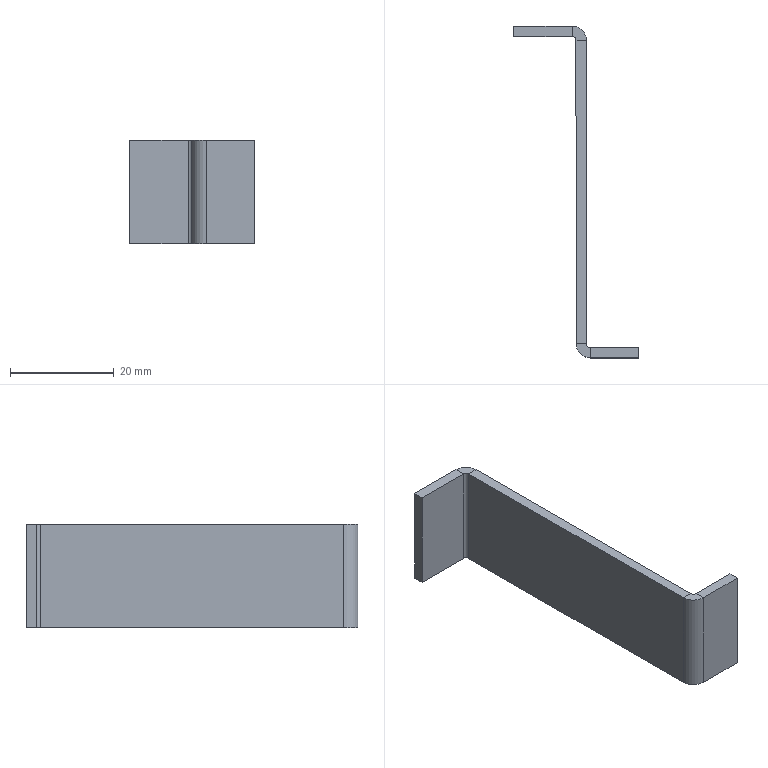Part | SolidWorks | features FlatPattern 1, SMBaseFlange 1, SheetMetal 1 | 1 solid | 22 faces | box 24 x 64 x 20 mm | volume 3380 mm3 | plane 18 | cylinder 4 | commonest cylinder face diameters 1.473 x2 5.473 x2
STEP:
#1=CARTESIAN_POINT('',(14.,-2.737,10.));
#2=VERTEX_POINT('',#1);
#3=CARTESIAN_POINT('',(12.,-2.737,10.));
#4=VERTEX_POINT('',#3);
#5=CARTESIAN_POINT('',(14.,-2.737,10.));
#6=DIRECTION('',(-1.,0.,0.));
#7=VECTOR('',#6,1000.);
#8=LINE('',#5,#7);
#9=EDGE_CURVE('',#2,#4,#8,.T.);
#10=ORIENTED_EDGE('',*,*,#9,.F.);
#11=CARTESIAN_POINT('',(11.263,0.,10.));
#12=VERTEX_POINT('',#11);
#13=CARTESIAN_POINT('',(11.263,-2.737,10.));
#14=DIRECTION('',(0.,0.,-1.));
#15=DIRECTION('',(1.,0.,0.));
#16=AXIS2_PLACEMENT_3D('',#13,#14,#15);
#17=CIRCLE('',#16,2.737);
#18=EDGE_CURVE('',#12,#2,#17,.T.);
#19=ORIENTED_EDGE('',*,*,#18,.F.);
#20=CARTESIAN_POINT('',(11.263,-2.,10.));
#21=VERTEX_POINT('',#20);
#22=CARTESIAN_POINT('',(11.263,-2.,10.));
#23=DIRECTION('',(0.,1.,0.));
#24=VECTOR('',#23,1000.);
#25=LINE('',#22,#24);
#26=EDGE_CURVE('',#21,#12,#25,.T.);
#27=ORIENTED_EDGE('',*,*,#26,.F.);
#28=CARTESIAN_POINT('',(11.263,-2.737,10.));
#29=DIRECTION('',(0.,0.,-1.));
#30=DIRECTION('',(1.,0.,0.));
#31=AXIS2_PLACEMENT_3D('',#28,#29,#30);
#32=CIRCLE('',#31,0.7366);
#33=EDGE_CURVE('',#21,#4,#32,.T.);
#34=ORIENTED_EDGE('',*,*,#33,.T.);
#35=EDGE_LOOP('',(#10,#19,#27,#34));
#36=FACE_OUTER_BOUND('',#35,.T.);
#37=CARTESIAN_POINT('',(14.,-2.737,10.));
#38=DIRECTION('',(0.,0.,1.));
#39=DIRECTION('',(1.,0.,0.));
#40=AXIS2_PLACEMENT_3D('',#37,#38,#39);
#41=PLANE('',#40);
#42=ADVANCED_FACE('',(#36),#41,.T.);
#43=CARTESIAN_POINT('',(14.,-61.263,10.));
#44=VERTEX_POINT('',#43);
#45=CARTESIAN_POINT('',(14.,0.,10.));
#46=DIRECTION('',(0.,-1.,0.));
#47=VECTOR('',#46,1000.);
#48=LINE('',#45,#47);
#49=EDGE_CURVE('',#2,#44,#48,.T.);
#50=ORIENTED_EDGE('',*,*,#49,.F.);
#51=ORIENTED_EDGE('',*,*,#9,.T.);
#52=CARTESIAN_POINT('',(12.,-61.263,10.));
#53=VERTEX_POINT('',#52);
#54=CARTESIAN_POINT('',(12.,0.,10.));
#55=DIRECTION('',(0.,-1.,0.));
#56=VECTOR('',#55,1000.);
#57=LINE('',#54,#56);
#58=EDGE_CURVE('',#4,#53,#57,.T.);
#59=ORIENTED_EDGE('',*,*,#58,.T.);
#60=CARTESIAN_POINT('',(12.,-61.263,10.));
#61=DIRECTION('',(1.,0.,0.));
#62=VECTOR('',#61,1000.);
#63=LINE('',#60,#62);
#64=EDGE_CURVE('',#53,#44,#63,.T.);
#65=ORIENTED_EDGE('',*,*,#64,.T.);
#66=EDGE_LOOP('',(#50,#51,#59,#65));
#67=FACE_OUTER_BOUND('',#66,.T.);
#68=CARTESIAN_POINT('',(11.263,-2.,10.));
#69=DIRECTION('',(0.,0.,1.));
#70=DIRECTION('',(1.,0.,0.));
#71=AXIS2_PLACEMENT_3D('',#68,#69,#70);
#72=PLANE('',#71);
#73=ADVANCED_FACE('',(#67),#72,.T.);
#74=CARTESIAN_POINT('',(11.263,0.,-10.));
#75=VERTEX_POINT('',#74);
#76=CARTESIAN_POINT('',(11.263,-2.,-10.));
#77=VERTEX_POINT('',#76);
#78=CARTESIAN_POINT('',(11.263,0.,-10.));
#79=DIRECTION('',(0.,-1.,0.));
#80=VECTOR('',#79,1000.);
#81=LINE('',#78,#80);
#82=EDGE_CURVE('',#75,#77,#81,.T.);
#83=ORIENTED_EDGE('',*,*,#82,.F.);
#84=CARTESIAN_POINT('',(14.,-2.737,-10.));
#85=VERTEX_POINT('',#84);
#86=CARTESIAN_POINT('',(11.263,-2.737,-10.));
#87=DIRECTION('',(0.,0.,-1.));
#88=DIRECTION('',(1.,0.,0.));
#89=AXIS2_PLACEMENT_3D('',#86,#87,#88);
#90=CIRCLE('',#89,2.737);
#91=EDGE_CURVE('',#75,#85,#90,.T.);
#92=ORIENTED_EDGE('',*,*,#91,.T.);
#93=CARTESIAN_POINT('',(12.,-2.737,-10.));
#94=VERTEX_POINT('',#93);
#95=CARTESIAN_POINT('',(12.,-2.737,-10.));
#96=DIRECTION('',(1.,0.,0.));
#97=VECTOR('',#96,1000.);
#98=LINE('',#95,#97);
#99=EDGE_CURVE('',#94,#85,#98,.T.);
#100=ORIENTED_EDGE('',*,*,#99,.F.);
#101=CARTESIAN_POINT('',(11.263,-2.737,-10.));
#102=DIRECTION('',(0.,0.,-1.));
#103=DIRECTION('',(1.,0.,0.));
#104=AXIS2_PLACEMENT_3D('',#101,#102,#103);
#105=CIRCLE('',#104,0.7366);
#106=EDGE_CURVE('',#77,#94,#105,.T.);
#107=ORIENTED_EDGE('',*,*,#106,.F.);
#108=EDGE_LOOP('',(#83,#92,#100,#107));
#109=FACE_OUTER_BOUND('',#108,.T.);
#110=CARTESIAN_POINT('',(11.263,0.,-10.));
#111=DIRECTION('',(0.,0.,-1.));
#112=DIRECTION('',(-1.,0.,0.));
#113=AXIS2_PLACEMENT_3D('',#110,#111,#112);
#114=PLANE('',#113);
#115=ADVANCED_FACE('',(#109),#114,.T.);
#116=CARTESIAN_POINT('',(0.,0.,-10.));
#117=VERTEX_POINT('',#116);
#118=CARTESIAN_POINT('',(0.,0.,-10.));
#119=DIRECTION('',(1.,0.,0.));
#120=VECTOR('',#119,1000.);
#121=LINE('',#118,#120);
#122=EDGE_CURVE('',#117,#75,#121,.T.);
#123=ORIENTED_EDGE('',*,*,#122,.T.);
#124=ORIENTED_EDGE('',*,*,#82,.T.);
#125=CARTESIAN_POINT('',(0.,-2.,-10.));
#126=VERTEX_POINT('',#125);
#127=CARTESIAN_POINT('',(0.,-2.,-10.));
#128=DIRECTION('',(1.,0.,0.));
#129=VECTOR('',#128,1000.);
#130=LINE('',#127,#129);
#131=EDGE_CURVE('',#126,#77,#130,.T.);
#132=ORIENTED_EDGE('',*,*,#131,.F.);
#133=CARTESIAN_POINT('',(0.,-2.,-10.));
#134=DIRECTION('',(0.,1.,0.));
#135=VECTOR('',#134,1000.);
#136=LINE('',#133,#135);
#137=EDGE_CURVE('',#126,#117,#136,.T.);
#138=ORIENTED_EDGE('',*,*,#137,.T.);
#139=EDGE_LOOP('',(#123,#124,#132,#138));
#140=FACE_OUTER_BOUND('',#139,.T.);
#141=CARTESIAN_POINT('',(12.,-2.737,-10.));
#142=DIRECTION('',(0.,0.,-1.));
#143=DIRECTION('',(-1.,0.,0.));
#144=AXIS2_PLACEMENT_3D('',#141,#142,#143);
#145=PLANE('',#144);
#146=ADVANCED_FACE('',(#140),#145,.T.);
#147=CARTESIAN_POINT('',(14.737,-62.,10.));
#148=VERTEX_POINT('',#147);
#149=CARTESIAN_POINT('',(14.737,-64.,10.));
#150=VERTEX_POINT('',#149);
#151=CARTESIAN_POINT('',(14.737,-62.,10.));
#152=DIRECTION('',(0.,-1.,0.));
#153=VECTOR('',#152,1000.);
#154=LINE('',#151,#153);
#155=EDGE_CURVE('',#148,#150,#154,.T.);
#156=ORIENTED_EDGE('',*,*,#155,.F.);
#157=CARTESIAN_POINT('',(14.737,-61.263,10.));
#158=DIRECTION('',(0.,0.,1.));
#159=DIRECTION('',(-1.,0.,0.));
#160=AXIS2_PLACEMENT_3D('',#157,#158,#159);
#161=CIRCLE('',#160,0.7366);
#162=EDGE_CURVE('',#44,#148,#161,.T.);
#163=ORIENTED_EDGE('',*,*,#162,.F.);
#164=ORIENTED_EDGE('',*,*,#64,.F.);
#165=CARTESIAN_POINT('',(14.737,-61.263,10.));
#166=DIRECTION('',(0.,0.,1.));
#167=DIRECTION('',(1.,0.,0.));
#168=AXIS2_PLACEMENT_3D('',#165,#166,#167);
#169=CIRCLE('',#168,2.737);
#170=EDGE_CURVE('',#53,#150,#169,.T.);
#171=ORIENTED_EDGE('',*,*,#170,.T.);
#172=EDGE_LOOP('',(#156,#163,#164,#171));
#173=FACE_OUTER_BOUND('',#172,.T.);
#174=CARTESIAN_POINT('',(14.737,-62.,10.));
#175=DIRECTION('',(0.,0.,1.));
#176=DIRECTION('',(1.,0.,0.));
#177=AXIS2_PLACEMENT_3D('',#174,#175,#176);
#178=PLANE('',#177);
#179=ADVANCED_FACE('',(#173),#178,.T.);
#180=CARTESIAN_POINT('',(24.,-62.,10.));
#181=VERTEX_POINT('',#180);
#182=CARTESIAN_POINT('',(14.,-62.,10.));
#183=DIRECTION('',(1.,0.,0.));
#184=VECTOR('',#183,1000.);
#185=LINE('',#182,#184);
#186=EDGE_CURVE('',#148,#181,#185,.T.);
#187=ORIENTED_EDGE('',*,*,#186,.F.);
#188=ORIENTED_EDGE('',*,*,#155,.T.);
#189=CARTESIAN_POINT('',(24.,-64.,10.));
#190=VERTEX_POINT('',#189);
#191=CARTESIAN_POINT('',(14.,-64.,10.));
#192=DIRECTION('',(1.,0.,0.));
#193=VECTOR('',#192,1000.);
#194=LINE('',#191,#193);
#195=EDGE_CURVE('',#150,#190,#194,.T.);
#196=ORIENTED_EDGE('',*,*,#195,.T.);
#197=CARTESIAN_POINT('',(24.,-62.,10.));
#198=DIRECTION('',(0.,-1.,0.));
#199=VECTOR('',#198,1000.);
#200=LINE('',#197,#199);
#201=EDGE_CURVE('',#181,#190,#200,.T.);
#202=ORIENTED_EDGE('',*,*,#201,.F.);
#203=EDGE_LOOP('',(#187,#188,#196,#202));
#204=FACE_OUTER_BOUND('',#203,.T.);
#205=CARTESIAN_POINT('',(12.,-61.263,10.));
#206=DIRECTION('',(0.,0.,1.));
#207=DIRECTION('',(1.,0.,0.));
#208=AXIS2_PLACEMENT_3D('',#205,#206,#207);
#209=PLANE('',#208);
#210=ADVANCED_FACE('',(#204),#209,.T.);
#211=CARTESIAN_POINT('',(14.,-61.263,-10.));
#212=VERTEX_POINT('',#211);
#213=CARTESIAN_POINT('',(12.,-61.263,-10.));
#214=VERTEX_POINT('',#213);
#215=CARTESIAN_POINT('',(14.,-61.263,-10.));
#216=DIRECTION('',(-1.,0.,0.));
#217=VECTOR('',#216,1000.);
#218=LINE('',#215,#217);
#219=EDGE_CURVE('',#212,#214,#218,.T.);
#220=ORIENTED_EDGE('',*,*,#219,.F.);
#221=CARTESIAN_POINT('',(14.737,-62.,-10.));
#222=VERTEX_POINT('',#221);
#223=CARTESIAN_POINT('',(14.737,-61.263,-10.));
#224=DIRECTION('',(0.,0.,1.));
#225=DIRECTION('',(-1.,0.,0.));
#226=AXIS2_PLACEMENT_3D('',#223,#224,#225);
#227=CIRCLE('',#226,0.7366);
#228=EDGE_CURVE('',#212,#222,#227,.T.);
#229=ORIENTED_EDGE('',*,*,#228,.T.);
#230=CARTESIAN_POINT('',(14.737,-64.,-10.));
#231=VERTEX_POINT('',#230);
#232=CARTESIAN_POINT('',(14.737,-64.,-10.));
#233=DIRECTION('',(0.,1.,0.));
#234=VECTOR('',#233,1000.);
#235=LINE('',#232,#234);
#236=EDGE_CURVE('',#231,#222,#235,.T.);
#237=ORIENTED_EDGE('',*,*,#236,.F.);
#238=CARTESIAN_POINT('',(14.737,-61.263,-10.));
#239=DIRECTION('',(0.,0.,1.));
#240=DIRECTION('',(1.,0.,0.));
#241=AXIS2_PLACEMENT_3D('',#238,#239,#240);
#242=CIRCLE('',#241,2.737);
#243=EDGE_CURVE('',#214,#231,#242,.T.);
#244=ORIENTED_EDGE('',*,*,#243,.F.);
#245=EDGE_LOOP('',(#220,#229,#237,#244));
#246=FACE_OUTER_BOUND('',#245,.T.);
#247=CARTESIAN_POINT('',(14.,-61.263,-10.));
#248=DIRECTION('',(0.,0.,-1.));
#249=DIRECTION('',(-1.,0.,0.));
#250=AXIS2_PLACEMENT_3D('',#247,#248,#249);
#251=PLANE('',#250);
#252=ADVANCED_FACE('',(#246),#251,.T.);
#253=CARTESIAN_POINT('',(14.,0.,-10.));
#254=DIRECTION('',(0.,-1.,0.));
#255=VECTOR('',#254,1000.);
#256=LINE('',#253,#255);
#257=EDGE_CURVE('',#85,#212,#256,.T.);
#258=ORIENTED_EDGE('',*,*,#257,.T.);
#259=ORIENTED_EDGE('',*,*,#219,.T.);
#260=CARTESIAN_POINT('',(12.,0.,-10.));
#261=DIRECTION('',(0.,-1.,0.));
#262=VECTOR('',#261,1000.);
#263=LINE('',#260,#262);
#264=EDGE_CURVE('',#94,#214,#263,.T.);
#265=ORIENTED_EDGE('',*,*,#264,.F.);
#266=ORIENTED_EDGE('',*,*,#99,.T.);
#267=EDGE_LOOP('',(#258,#259,#265,#266));
#268=FACE_OUTER_BOUND('',#267,.T.);
#269=CARTESIAN_POINT('',(14.737,-64.,-10.));
#270=DIRECTION('',(0.,0.,-1.));
#271=DIRECTION('',(-1.,0.,0.));
#272=AXIS2_PLACEMENT_3D('',#269,#270,#271);
#273=PLANE('',#272);
#274=ADVANCED_FACE('',(#268),#273,.T.);
#275=CARTESIAN_POINT('',(24.,-64.,-10.));
#276=VERTEX_POINT('',#275);
#277=CARTESIAN_POINT('',(14.,-64.,-10.));
#278=DIRECTION('',(1.,0.,0.));
#279=VECTOR('',#278,1000.);
#280=LINE('',#277,#279);
#281=EDGE_CURVE('',#231,#276,#280,.T.);
#282=ORIENTED_EDGE('',*,*,#281,.T.);
#283=CARTESIAN_POINT('',(24.,-64.,10.));
#284=DIRECTION('',(0.,0.,-1.));
#285=VECTOR('',#284,1000.);
#286=LINE('',#283,#285);
#287=EDGE_CURVE('',#190,#276,#286,.T.);
#288=ORIENTED_EDGE('',*,*,#287,.F.);
#289=ORIENTED_EDGE('',*,*,#195,.F.);
#290=CARTESIAN_POINT('',(14.737,-64.,10.));
#291=DIRECTION('',(0.,0.,-1.));
#292=VECTOR('',#291,1000.);
#293=LINE('',#290,#292);
#294=EDGE_CURVE('',#150,#231,#293,.T.);
#295=ORIENTED_EDGE('',*,*,#294,.T.);
#296=EDGE_LOOP('',(#282,#288,#289,#295));
#297=FACE_OUTER_BOUND('',#296,.T.);
#298=CARTESIAN_POINT('',(14.,-64.,10.));
#299=DIRECTION('',(0.,1.,0.));
#300=DIRECTION('',(0.,0.,1.));
#301=AXIS2_PLACEMENT_3D('',#298,#299,#300);
#302=PLANE('',#301);
#303=ADVANCED_FACE('',(#297),#302,.F.);
#304=CARTESIAN_POINT('',(24.,-62.,-10.));
#305=VERTEX_POINT('',#304);
#306=CARTESIAN_POINT('',(24.,-62.,-10.));
#307=DIRECTION('',(0.,-1.,0.));
#308=VECTOR('',#307,1000.);
#309=LINE('',#306,#308);
#310=EDGE_CURVE('',#305,#276,#309,.T.);
#311=ORIENTED_EDGE('',*,*,#310,.F.);
#312=CARTESIAN_POINT('',(24.,-62.,10.));
#313=DIRECTION('',(0.,0.,-1.));
#314=VECTOR('',#313,1000.);
#315=LINE('',#312,#314);
#316=EDGE_CURVE('',#181,#305,#315,.T.);
#317=ORIENTED_EDGE('',*,*,#316,.F.);
#318=ORIENTED_EDGE('',*,*,#201,.T.);
#319=ORIENTED_EDGE('',*,*,#287,.T.);
#320=EDGE_LOOP('',(#311,#317,#318,#319));
#321=FACE_OUTER_BOUND('',#320,.T.);
#322=CARTESIAN_POINT('',(24.,-62.,10.));
#323=DIRECTION('',(1.,0.,0.));
#324=DIRECTION('',(0.,0.,-1.));
#325=AXIS2_PLACEMENT_3D('',#322,#323,#324);
#326=PLANE('',#325);
#327=ADVANCED_FACE('',(#321),#326,.T.);
#328=CARTESIAN_POINT('',(14.,-62.,-10.));
#329=DIRECTION('',(1.,0.,0.));
#330=VECTOR('',#329,1000.);
#331=LINE('',#328,#330);
#332=EDGE_CURVE('',#222,#305,#331,.T.);
#333=ORIENTED_EDGE('',*,*,#332,.F.);
#334=CARTESIAN_POINT('',(14.737,-62.,10.));
#335=DIRECTION('',(0.,0.,-1.));
#336=VECTOR('',#335,1000.);
#337=LINE('',#334,#336);
#338=EDGE_CURVE('',#148,#222,#337,.T.);
#339=ORIENTED_EDGE('',*,*,#338,.F.);
#340=ORIENTED_EDGE('',*,*,#186,.T.);
#341=ORIENTED_EDGE('',*,*,#316,.T.);
#342=EDGE_LOOP('',(#333,#339,#340,#341));
#343=FACE_OUTER_BOUND('',#342,.T.);
#344=CARTESIAN_POINT('',(14.,-62.,10.));
#345=DIRECTION('',(0.,1.,0.));
#346=DIRECTION('',(0.,0.,1.));
#347=AXIS2_PLACEMENT_3D('',#344,#345,#346);
#348=PLANE('',#347);
#349=ADVANCED_FACE('',(#343),#348,.T.);
#350=ORIENTED_EDGE('',*,*,#228,.F.);
#351=CARTESIAN_POINT('',(14.,-61.263,10.));
#352=DIRECTION('',(0.,0.,-1.));
#353=VECTOR('',#352,1000.);
#354=LINE('',#351,#353);
#355=EDGE_CURVE('',#44,#212,#354,.T.);
#356=ORIENTED_EDGE('',*,*,#355,.F.);
#357=ORIENTED_EDGE('',*,*,#162,.T.);
#358=ORIENTED_EDGE('',*,*,#338,.T.);
#359=EDGE_LOOP('',(#350,#356,#357,#358));
#360=FACE_OUTER_BOUND('',#359,.T.);
#361=CARTESIAN_POINT('',(14.737,-61.263,10.));
#362=DIRECTION('',(0.,0.,-1.));
#363=DIRECTION('',(-1.,0.,0.));
#364=AXIS2_PLACEMENT_3D('',#361,#362,#363);
#365=CYLINDRICAL_SURFACE('',#364,0.7366);
#366=ADVANCED_FACE('',(#360),#365,.F.);
#367=ORIENTED_EDGE('',*,*,#257,.F.);
#368=CARTESIAN_POINT('',(14.,-2.737,10.));
#369=DIRECTION('',(0.,0.,-1.));
#370=VECTOR('',#369,1000.);
#371=LINE('',#368,#370);
#372=EDGE_CURVE('',#2,#85,#371,.T.);
#373=ORIENTED_EDGE('',*,*,#372,.F.);
#374=ORIENTED_EDGE('',*,*,#49,.T.);
#375=ORIENTED_EDGE('',*,*,#355,.T.);
#376=EDGE_LOOP('',(#367,#373,#374,#375));
#377=FACE_OUTER_BOUND('',#376,.T.);
#378=CARTESIAN_POINT('',(14.,0.,10.));
#379=DIRECTION('',(1.,0.,0.));
#380=DIRECTION('',(0.,1.,0.));
#381=AXIS2_PLACEMENT_3D('',#378,#379,#380);
#382=PLANE('',#381);
#383=ADVANCED_FACE('',(#377),#382,.T.);
#384=ORIENTED_EDGE('',*,*,#91,.F.);
#385=CARTESIAN_POINT('',(11.263,0.,10.));
#386=DIRECTION('',(0.,0.,-1.));
#387=VECTOR('',#386,1000.);
#388=LINE('',#385,#387);
#389=EDGE_CURVE('',#12,#75,#388,.T.);
#390=ORIENTED_EDGE('',*,*,#389,.F.);
#391=ORIENTED_EDGE('',*,*,#18,.T.);
#392=ORIENTED_EDGE('',*,*,#372,.T.);
#393=EDGE_LOOP('',(#384,#390,#391,#392));
#394=FACE_OUTER_BOUND('',#393,.T.);
#395=CARTESIAN_POINT('',(11.263,-2.737,10.));
#396=DIRECTION('',(0.,0.,-1.));
#397=DIRECTION('',(-1.,0.,0.));
#398=AXIS2_PLACEMENT_3D('',#395,#396,#397);
#399=CYLINDRICAL_SURFACE('',#398,2.737);
#400=ADVANCED_FACE('',(#394),#399,.T.);
#401=ORIENTED_EDGE('',*,*,#122,.F.);
#402=CARTESIAN_POINT('',(0.,0.,10.));
#403=VERTEX_POINT('',#402);
#404=CARTESIAN_POINT('',(0.,0.,10.));
#405=DIRECTION('',(0.,0.,-1.));
#406=VECTOR('',#405,1000.);
#407=LINE('',#404,#406);
#408=EDGE_CURVE('',#403,#117,#407,.T.);
#409=ORIENTED_EDGE('',*,*,#408,.F.);
#410=CARTESIAN_POINT('',(0.,0.,10.));
#411=DIRECTION('',(1.,0.,0.));
#412=VECTOR('',#411,1000.);
#413=LINE('',#410,#412);
#414=EDGE_CURVE('',#403,#12,#413,.T.);
#415=ORIENTED_EDGE('',*,*,#414,.T.);
#416=ORIENTED_EDGE('',*,*,#389,.T.);
#417=EDGE_LOOP('',(#401,#409,#415,#416));
#418=FACE_OUTER_BOUND('',#417,.T.);
#419=CARTESIAN_POINT('',(0.,0.,10.));
#420=DIRECTION('',(0.,1.,0.));
#421=DIRECTION('',(0.,0.,1.));
#422=AXIS2_PLACEMENT_3D('',#419,#420,#421);
#423=PLANE('',#422);
#424=ADVANCED_FACE('',(#418),#423,.T.);
#425=ORIENTED_EDGE('',*,*,#137,.F.);
#426=CARTESIAN_POINT('',(0.,-2.,10.));
#427=VERTEX_POINT('',#426);
#428=CARTESIAN_POINT('',(0.,-2.,10.));
#429=DIRECTION('',(0.,0.,-1.));
#430=VECTOR('',#429,1000.);
#431=LINE('',#428,#430);
#432=EDGE_CURVE('',#427,#126,#431,.T.);
#433=ORIENTED_EDGE('',*,*,#432,.F.);
#434=CARTESIAN_POINT('',(0.,-2.,10.));
#435=DIRECTION('',(0.,1.,0.));
#436=VECTOR('',#435,1000.);
#437=LINE('',#434,#436);
#438=EDGE_CURVE('',#427,#403,#437,.T.);
#439=ORIENTED_EDGE('',*,*,#438,.T.);
#440=ORIENTED_EDGE('',*,*,#408,.T.);
#441=EDGE_LOOP('',(#425,#433,#439,#440));
#442=FACE_OUTER_BOUND('',#441,.T.);
#443=CARTESIAN_POINT('',(0.,-2.,10.));
#444=DIRECTION('',(-1.,0.,0.));
#445=DIRECTION('',(0.,0.,1.));
#446=AXIS2_PLACEMENT_3D('',#443,#444,#445);
#447=PLANE('',#446);
#448=ADVANCED_FACE('',(#442),#447,.T.);
#449=ORIENTED_EDGE('',*,*,#131,.T.);
#450=CARTESIAN_POINT('',(11.263,-2.,10.));
#451=DIRECTION('',(0.,0.,-1.));
#452=VECTOR('',#451,1000.);
#453=LINE('',#450,#452);
#454=EDGE_CURVE('',#21,#77,#453,.T.);
#455=ORIENTED_EDGE('',*,*,#454,.F.);
#456=CARTESIAN_POINT('',(0.,-2.,10.));
#457=DIRECTION('',(1.,0.,0.));
#458=VECTOR('',#457,1000.);
#459=LINE('',#456,#458);
#460=EDGE_CURVE('',#427,#21,#459,.T.);
#461=ORIENTED_EDGE('',*,*,#460,.F.);
#462=ORIENTED_EDGE('',*,*,#432,.T.);
#463=EDGE_LOOP('',(#449,#455,#461,#462));
#464=FACE_OUTER_BOUND('',#463,.T.);
#465=CARTESIAN_POINT('',(0.,-2.,10.));
#466=DIRECTION('',(0.,1.,0.));
#467=DIRECTION('',(0.,0.,1.));
#468=AXIS2_PLACEMENT_3D('',#465,#466,#467);
#469=PLANE('',#468);
#470=ADVANCED_FACE('',(#464),#469,.F.);
#471=ORIENTED_EDGE('',*,*,#106,.T.);
#472=CARTESIAN_POINT('',(12.,-2.737,10.));
#473=DIRECTION('',(0.,0.,-1.));
#474=VECTOR('',#473,1000.);
#475=LINE('',#472,#474);
#476=EDGE_CURVE('',#4,#94,#475,.T.);
#477=ORIENTED_EDGE('',*,*,#476,.F.);
#478=ORIENTED_EDGE('',*,*,#33,.F.);
#479=ORIENTED_EDGE('',*,*,#454,.T.);
#480=EDGE_LOOP('',(#471,#477,#478,#479));
#481=FACE_OUTER_BOUND('',#480,.T.);
#482=CARTESIAN_POINT('',(11.263,-2.737,10.));
#483=DIRECTION('',(0.,0.,-1.));
#484=DIRECTION('',(-1.,0.,0.));
#485=AXIS2_PLACEMENT_3D('',#482,#483,#484);
#486=CYLINDRICAL_SURFACE('',#485,0.7366);
#487=ADVANCED_FACE('',(#481),#486,.F.);
#488=ORIENTED_EDGE('',*,*,#264,.T.);
#489=CARTESIAN_POINT('',(12.,-61.263,10.));
#490=DIRECTION('',(0.,0.,-1.));
#491=VECTOR('',#490,1000.);
#492=LINE('',#489,#491);
#493=EDGE_CURVE('',#53,#214,#492,.T.);
#494=ORIENTED_EDGE('',*,*,#493,.F.);
#495=ORIENTED_EDGE('',*,*,#58,.F.);
#496=ORIENTED_EDGE('',*,*,#476,.T.);
#497=EDGE_LOOP('',(#488,#494,#495,#496));
#498=FACE_OUTER_BOUND('',#497,.T.);
#499=CARTESIAN_POINT('',(12.,0.,10.));
#500=DIRECTION('',(1.,0.,0.));
#501=DIRECTION('',(0.,1.,0.));
#502=AXIS2_PLACEMENT_3D('',#499,#500,#501);
#503=PLANE('',#502);
#504=ADVANCED_FACE('',(#498),#503,.F.);
#505=ORIENTED_EDGE('',*,*,#243,.T.);
#506=ORIENTED_EDGE('',*,*,#294,.F.);
#507=ORIENTED_EDGE('',*,*,#170,.F.);
#508=ORIENTED_EDGE('',*,*,#493,.T.);
#509=EDGE_LOOP('',(#505,#506,#507,#508));
#510=FACE_OUTER_BOUND('',#509,.T.);
#511=CARTESIAN_POINT('',(14.737,-61.263,10.));
#512=DIRECTION('',(0.,0.,-1.));
#513=DIRECTION('',(-1.,0.,0.));
#514=AXIS2_PLACEMENT_3D('',#511,#512,#513);
#515=CYLINDRICAL_SURFACE('',#514,2.737);
#516=ADVANCED_FACE('',(#510),#515,.T.);
#517=ORIENTED_EDGE('',*,*,#460,.T.);
#518=ORIENTED_EDGE('',*,*,#26,.T.);
#519=ORIENTED_EDGE('',*,*,#414,.F.);
#520=ORIENTED_EDGE('',*,*,#438,.F.);
#521=EDGE_LOOP('',(#517,#518,#519,#520));
#522=FACE_OUTER_BOUND('',#521,.T.);
#523=CARTESIAN_POINT('',(14.737,-61.263,10.));
#524=DIRECTION('',(0.,0.,-1.));
#525=DIRECTION('',(-1.,0.,0.));
#526=AXIS2_PLACEMENT_3D('',#523,#524,#525);
#527=PLANE('',#526);
#528=ADVANCED_FACE('',(#522),#527,.F.);
#529=ORIENTED_EDGE('',*,*,#281,.F.);
#530=ORIENTED_EDGE('',*,*,#236,.T.);
#531=ORIENTED_EDGE('',*,*,#332,.T.);
#532=ORIENTED_EDGE('',*,*,#310,.T.);
#533=EDGE_LOOP('',(#529,#530,#531,#532));
#534=FACE_OUTER_BOUND('',#533,.T.);
#535=CARTESIAN_POINT('',(14.737,-61.263,-10.));
#536=DIRECTION('',(0.,0.,-1.));
#537=DIRECTION('',(-1.,0.,0.));
#538=AXIS2_PLACEMENT_3D('',#535,#536,#537);
#539=PLANE('',#538);
#540=ADVANCED_FACE('',(#534),#539,.T.);
#541=CLOSED_SHELL('',(#42,#73,#115,#146,#179,#210,#252,#274,#303,#327,#349,#366,#383,#400,#424,#448,#470,#487,#504,#516,#528,#540));
#542=MANIFOLD_SOLID_BREP('',#541);
#543=CARTESIAN_POINT('',(0.,0.,0.));
#544=DIRECTION('',(0.,0.,1.));
#545=DIRECTION('',(1.,0.,0.));
#546=AXIS2_PLACEMENT_3D('',#543,#544,#545);
#547=(LENGTH_UNIT()NAMED_UNIT(*)SI_UNIT(.MILLI.,.METRE.));
#548=UNCERTAINTY_MEASURE_WITH_UNIT(LENGTH_MEASURE(0.00001),#547,'','');
#549=(NAMED_UNIT(*)PLANE_ANGLE_UNIT()SI_UNIT($,.RADIAN.));
#550=(NAMED_UNIT(*)SI_UNIT($,.STERADIAN.)SOLID_ANGLE_UNIT());
#551=(GEOMETRIC_REPRESENTATION_CONTEXT(3)GLOBAL_UNCERTAINTY_ASSIGNED_CONTEXT((#548))GLOBAL_UNIT_ASSIGNED_CONTEXT((#547,#549,#550))REPRESENTATION_CONTEXT('',''));
#552=ADVANCED_BREP_SHAPE_REPRESENTATION('',(#542,#546),#551);